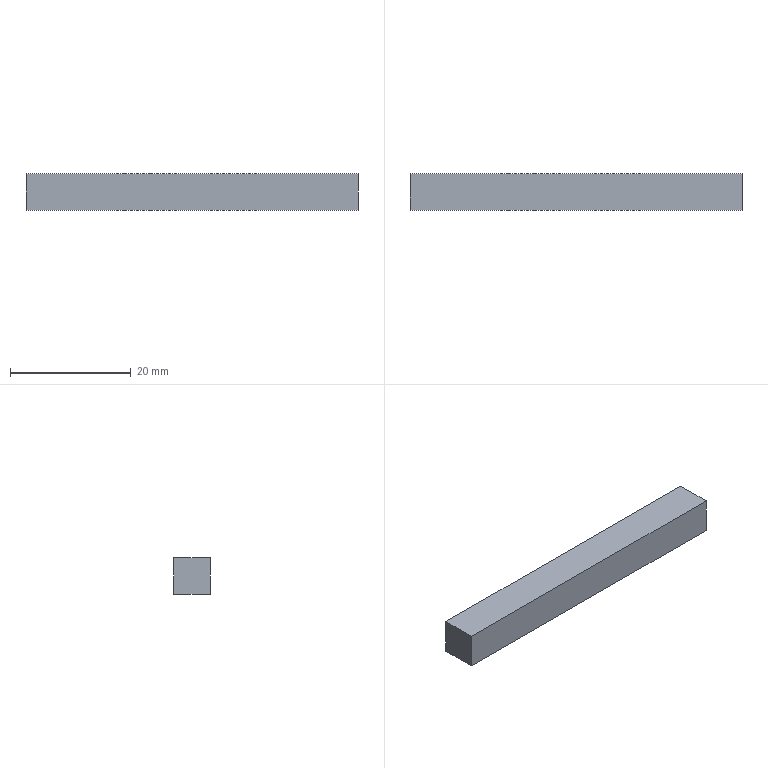Part | SolidWorks | features BaseBody 1 | 1 solid | 6 faces | box 55 x 6 x 6 mm | volume 1980 mm3 | plane 6
STEP:
#1=CARTESIAN_POINT('',(-27.5,6.,-3.));
#2=VERTEX_POINT('',#1);
#3=CARTESIAN_POINT('',(-27.5,0.,-3.));
#4=VERTEX_POINT('',#3);
#5=CARTESIAN_POINT('',(-27.5,6.,-3.));
#6=DIRECTION('',(0.,-1.,0.));
#7=VECTOR('',#6,1000.);
#8=LINE('',#5,#7);
#9=EDGE_CURVE('',#2,#4,#8,.T.);
#10=ORIENTED_EDGE('',*,*,#9,.F.);
#11=CARTESIAN_POINT('',(27.5,6.,-3.));
#12=VERTEX_POINT('',#11);
#13=CARTESIAN_POINT('',(-27.5,6.,-3.));
#14=DIRECTION('',(-1.,0.,0.));
#15=VECTOR('',#14,1000.);
#16=LINE('',#13,#15);
#17=EDGE_CURVE('',#12,#2,#16,.T.);
#18=ORIENTED_EDGE('',*,*,#17,.F.);
#19=CARTESIAN_POINT('',(27.5,0.,-3.));
#20=VERTEX_POINT('',#19);
#21=CARTESIAN_POINT('',(27.5,6.,-3.));
#22=DIRECTION('',(0.,1.,0.));
#23=VECTOR('',#22,1000.);
#24=LINE('',#21,#23);
#25=EDGE_CURVE('',#20,#12,#24,.T.);
#26=ORIENTED_EDGE('',*,*,#25,.F.);
#27=CARTESIAN_POINT('',(-27.5,0.,-3.));
#28=DIRECTION('',(1.,0.,0.));
#29=VECTOR('',#28,1000.);
#30=LINE('',#27,#29);
#31=EDGE_CURVE('',#4,#20,#30,.T.);
#32=ORIENTED_EDGE('',*,*,#31,.F.);
#33=EDGE_LOOP('',(#10,#18,#26,#32));
#34=FACE_OUTER_BOUND('',#33,.T.);
#35=CARTESIAN_POINT('',(-27.5,6.,-3.));
#36=DIRECTION('',(0.,0.,1.));
#37=DIRECTION('',(1.,0.,0.));
#38=AXIS2_PLACEMENT_3D('',#35,#36,#37);
#39=PLANE('',#38);
#40=ADVANCED_FACE('',(#34),#39,.F.);
#41=CARTESIAN_POINT('',(-27.5,0.,3.));
#42=VERTEX_POINT('',#41);
#43=CARTESIAN_POINT('',(-27.5,0.,0.));
#44=DIRECTION('',(0.,0.,-1.));
#45=VECTOR('',#44,1000.);
#46=LINE('',#43,#45);
#47=EDGE_CURVE('',#42,#4,#46,.T.);
#48=ORIENTED_EDGE('',*,*,#47,.T.);
#49=ORIENTED_EDGE('',*,*,#31,.T.);
#50=CARTESIAN_POINT('',(27.5,0.,3.));
#51=VERTEX_POINT('',#50);
#52=CARTESIAN_POINT('',(27.5,0.,0.));
#53=DIRECTION('',(0.,0.,1.));
#54=VECTOR('',#53,1000.);
#55=LINE('',#52,#54);
#56=EDGE_CURVE('',#20,#51,#55,.T.);
#57=ORIENTED_EDGE('',*,*,#56,.T.);
#58=CARTESIAN_POINT('',(0.,0.,3.));
#59=DIRECTION('',(-1.,0.,0.));
#60=VECTOR('',#59,1000.);
#61=LINE('',#58,#60);
#62=EDGE_CURVE('',#51,#42,#61,.T.);
#63=ORIENTED_EDGE('',*,*,#62,.T.);
#64=EDGE_LOOP('',(#48,#49,#57,#63));
#65=FACE_OUTER_BOUND('',#64,.T.);
#66=CARTESIAN_POINT('',(0.,0.,0.));
#67=DIRECTION('',(0.,-1.,0.));
#68=DIRECTION('',(0.,0.,-1.));
#69=AXIS2_PLACEMENT_3D('',#66,#67,#68);
#70=PLANE('',#69);
#71=ADVANCED_FACE('',(#65),#70,.T.);
#72=CARTESIAN_POINT('',(-27.5,6.,3.));
#73=VERTEX_POINT('',#72);
#74=CARTESIAN_POINT('',(-27.5,6.,3.));
#75=DIRECTION('',(0.,-1.,0.));
#76=VECTOR('',#75,1000.);
#77=LINE('',#74,#76);
#78=EDGE_CURVE('',#73,#42,#77,.T.);
#79=ORIENTED_EDGE('',*,*,#78,.F.);
#80=CARTESIAN_POINT('',(-27.5,6.,3.));
#81=DIRECTION('',(0.,0.,1.));
#82=VECTOR('',#81,1000.);
#83=LINE('',#80,#82);
#84=EDGE_CURVE('',#2,#73,#83,.T.);
#85=ORIENTED_EDGE('',*,*,#84,.F.);
#86=ORIENTED_EDGE('',*,*,#9,.T.);
#87=ORIENTED_EDGE('',*,*,#47,.F.);
#88=EDGE_LOOP('',(#79,#85,#86,#87));
#89=FACE_OUTER_BOUND('',#88,.T.);
#90=CARTESIAN_POINT('',(-27.5,6.,3.));
#91=DIRECTION('',(1.,0.,0.));
#92=DIRECTION('',(0.,0.,-1.));
#93=AXIS2_PLACEMENT_3D('',#90,#91,#92);
#94=PLANE('',#93);
#95=ADVANCED_FACE('',(#89),#94,.F.);
#96=ORIENTED_EDGE('',*,*,#17,.T.);
#97=ORIENTED_EDGE('',*,*,#84,.T.);
#98=CARTESIAN_POINT('',(27.5,6.,3.));
#99=VERTEX_POINT('',#98);
#100=CARTESIAN_POINT('',(0.,6.,3.));
#101=DIRECTION('',(-1.,0.,0.));
#102=VECTOR('',#101,1000.);
#103=LINE('',#100,#102);
#104=EDGE_CURVE('',#99,#73,#103,.T.);
#105=ORIENTED_EDGE('',*,*,#104,.F.);
#106=CARTESIAN_POINT('',(27.5,6.,0.));
#107=DIRECTION('',(0.,0.,1.));
#108=VECTOR('',#107,1000.);
#109=LINE('',#106,#108);
#110=EDGE_CURVE('',#12,#99,#109,.T.);
#111=ORIENTED_EDGE('',*,*,#110,.F.);
#112=EDGE_LOOP('',(#96,#97,#105,#111));
#113=FACE_OUTER_BOUND('',#112,.T.);
#114=CARTESIAN_POINT('',(0.,6.,0.));
#115=DIRECTION('',(0.,-1.,0.));
#116=DIRECTION('',(0.,0.,-1.));
#117=AXIS2_PLACEMENT_3D('',#114,#115,#116);
#118=PLANE('',#117);
#119=ADVANCED_FACE('',(#113),#118,.F.);
#120=ORIENTED_EDGE('',*,*,#25,.T.);
#121=ORIENTED_EDGE('',*,*,#110,.T.);
#122=CARTESIAN_POINT('',(27.5,6.,3.));
#123=DIRECTION('',(0.,1.,0.));
#124=VECTOR('',#123,1000.);
#125=LINE('',#122,#124);
#126=EDGE_CURVE('',#51,#99,#125,.T.);
#127=ORIENTED_EDGE('',*,*,#126,.F.);
#128=ORIENTED_EDGE('',*,*,#56,.F.);
#129=EDGE_LOOP('',(#120,#121,#127,#128));
#130=FACE_OUTER_BOUND('',#129,.T.);
#131=CARTESIAN_POINT('',(27.5,6.,3.));
#132=DIRECTION('',(-1.,0.,0.));
#133=DIRECTION('',(0.,0.,1.));
#134=AXIS2_PLACEMENT_3D('',#131,#132,#133);
#135=PLANE('',#134);
#136=ADVANCED_FACE('',(#130),#135,.F.);
#137=ORIENTED_EDGE('',*,*,#126,.T.);
#138=ORIENTED_EDGE('',*,*,#104,.T.);
#139=ORIENTED_EDGE('',*,*,#78,.T.);
#140=ORIENTED_EDGE('',*,*,#62,.F.);
#141=EDGE_LOOP('',(#137,#138,#139,#140));
#142=FACE_OUTER_BOUND('',#141,.T.);
#143=CARTESIAN_POINT('',(-27.5,6.,3.));
#144=DIRECTION('',(0.,0.,-1.));
#145=DIRECTION('',(-1.,0.,0.));
#146=AXIS2_PLACEMENT_3D('',#143,#144,#145);
#147=PLANE('',#146);
#148=ADVANCED_FACE('',(#142),#147,.F.);
#149=CLOSED_SHELL('',(#40,#71,#95,#119,#136,#148));
#150=MANIFOLD_SOLID_BREP('',#149);
#151=CARTESIAN_POINT('',(0.,0.,0.));
#152=DIRECTION('',(0.,0.,1.));
#153=DIRECTION('',(1.,0.,0.));
#154=AXIS2_PLACEMENT_3D('',#151,#152,#153);
#155=(LENGTH_UNIT()NAMED_UNIT(*)SI_UNIT(.MILLI.,.METRE.));
#156=UNCERTAINTY_MEASURE_WITH_UNIT(LENGTH_MEASURE(0.00001),#155,'','');
#157=(NAMED_UNIT(*)PLANE_ANGLE_UNIT()SI_UNIT($,.RADIAN.));
#158=(NAMED_UNIT(*)SI_UNIT($,.STERADIAN.)SOLID_ANGLE_UNIT());
#159=(GEOMETRIC_REPRESENTATION_CONTEXT(3)GLOBAL_UNCERTAINTY_ASSIGNED_CONTEXT((#156))GLOBAL_UNIT_ASSIGNED_CONTEXT((#155,#157,#158))REPRESENTATION_CONTEXT('',''));
#160=ADVANCED_BREP_SHAPE_REPRESENTATION('',(#150,#154),#159);